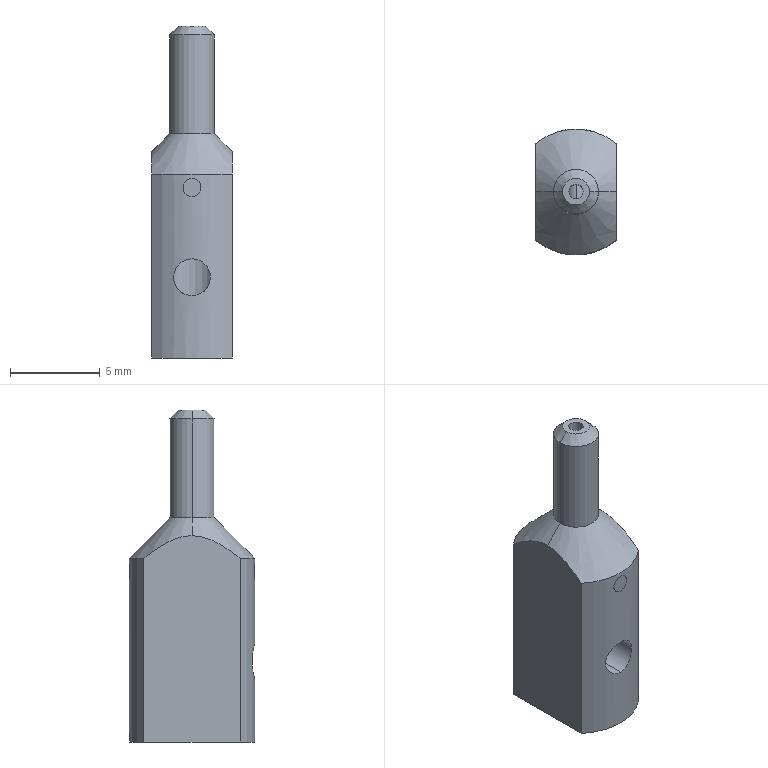Part | SolidWorks | features ICE 7, Chamfer 2, Extrusion 1, HoleWzd 1 | 2 solids | 27 faces | box 4.5 x 7 x 18.5 mm | volume 294.57 mm3 | cylinder 16 | plane 7 | cone 4 | commonest cylinder face diameters 0.8 x4 1 x4 2.05 x2 2.5 x2 3 x2 7 x2
STEP:
#1=CARTESIAN_POINT('',(0.,3.5,10.));
#2=VERTEX_POINT('',#1);
#3=CARTESIAN_POINT('',(0.,3.5,9.));
#4=VERTEX_POINT('',#3);
#5=CARTESIAN_POINT('',(0.,3.5,9.5));
#6=DIRECTION('',(0.,1.,0.));
#7=DIRECTION('',(0.,0.,1.));
#8=AXIS2_PLACEMENT_3D('',#5,#6,#7);
#9=CIRCLE('',#8,0.5);
#10=EDGE_CURVE('',#2,#4,#9,.T.);
#11=ORIENTED_EDGE('',*,*,#10,.F.);
#12=CARTESIAN_POINT('',(0.,-3.5,10.));
#13=VERTEX_POINT('',#12);
#14=CARTESIAN_POINT('',(0.,3.5,10.));
#15=DIRECTION('',(0.,-1.,0.));
#16=VECTOR('',#15,1000.);
#17=LINE('',#14,#16);
#18=EDGE_CURVE('',#2,#13,#17,.T.);
#19=ORIENTED_EDGE('',*,*,#18,.T.);
#20=CARTESIAN_POINT('',(0.,-3.5,9.));
#21=VERTEX_POINT('',#20);
#22=CARTESIAN_POINT('',(0.,-3.5,9.5));
#23=DIRECTION('',(0.,1.,0.));
#24=DIRECTION('',(0.,0.,1.));
#25=AXIS2_PLACEMENT_3D('',#22,#23,#24);
#26=CIRCLE('',#25,0.5);
#27=EDGE_CURVE('',#13,#21,#26,.T.);
#28=ORIENTED_EDGE('',*,*,#27,.T.);
#29=CARTESIAN_POINT('',(0.,3.5,9.));
#30=DIRECTION('',(0.,-1.,0.));
#31=VECTOR('',#30,1000.);
#32=LINE('',#29,#31);
#33=EDGE_CURVE('',#4,#21,#32,.T.);
#34=ORIENTED_EDGE('',*,*,#33,.F.);
#35=EDGE_LOOP('',(#11,#19,#28,#34));
#36=FACE_OUTER_BOUND('',#35,.T.);
#37=CARTESIAN_POINT('',(0.,3.5,9.5));
#38=DIRECTION('',(0.,-1.,0.));
#39=DIRECTION('',(0.,0.,-1.));
#40=AXIS2_PLACEMENT_3D('',#37,#38,#39);
#41=CYLINDRICAL_SURFACE('',#40,0.5);
#42=ADVANCED_FACE('',(#36),#41,.T.);
#43=ORIENTED_EDGE('',*,*,#18,.F.);
#44=CARTESIAN_POINT('',(0.,3.5,9.5));
#45=DIRECTION('',(0.,1.,0.));
#46=DIRECTION('',(0.,0.,1.));
#47=AXIS2_PLACEMENT_3D('',#44,#45,#46);
#48=CIRCLE('',#47,0.5);
#49=EDGE_CURVE('',#4,#2,#48,.T.);
#50=ORIENTED_EDGE('',*,*,#49,.F.);
#51=ORIENTED_EDGE('',*,*,#33,.T.);
#52=CARTESIAN_POINT('',(0.,-3.5,9.5));
#53=DIRECTION('',(0.,1.,0.));
#54=DIRECTION('',(0.,0.,1.));
#55=AXIS2_PLACEMENT_3D('',#52,#53,#54);
#56=CIRCLE('',#55,0.5);
#57=EDGE_CURVE('',#21,#13,#56,.T.);
#58=ORIENTED_EDGE('',*,*,#57,.T.);
#59=EDGE_LOOP('',(#43,#50,#51,#58));
#60=FACE_OUTER_BOUND('',#59,.T.);
#61=CARTESIAN_POINT('',(0.,3.5,9.5));
#62=DIRECTION('',(0.,-1.,0.));
#63=DIRECTION('',(0.,0.,-1.));
#64=AXIS2_PLACEMENT_3D('',#61,#62,#63);
#65=CYLINDRICAL_SURFACE('',#64,0.5);
#66=ADVANCED_FACE('',(#60),#65,.T.);
#67=ORIENTED_EDGE('',*,*,#49,.T.);
#68=ORIENTED_EDGE('',*,*,#10,.T.);
#69=EDGE_LOOP('',(#67,#68));
#70=FACE_OUTER_BOUND('',#69,.T.);
#71=CARTESIAN_POINT('',(0.,3.5,9.5));
#72=DIRECTION('',(0.,1.,0.));
#73=DIRECTION('',(0.,0.,1.));
#74=AXIS2_PLACEMENT_3D('',#71,#72,#73);
#75=PLANE('',#74);
#76=ADVANCED_FACE('',(#70),#75,.T.);
#77=ORIENTED_EDGE('',*,*,#57,.F.);
#78=ORIENTED_EDGE('',*,*,#27,.F.);
#79=EDGE_LOOP('',(#77,#78));
#80=FACE_OUTER_BOUND('',#79,.T.);
#81=CARTESIAN_POINT('',(0.,-3.5,9.5));
#82=DIRECTION('',(0.,1.,0.));
#83=DIRECTION('',(0.,0.,1.));
#84=AXIS2_PLACEMENT_3D('',#81,#82,#83);
#85=PLANE('',#84);
#86=ADVANCED_FACE('',(#80),#85,.F.);
#87=CLOSED_SHELL('',(#42,#66,#76,#86));
#88=MANIFOLD_SOLID_BREP('',#87);
#89=CARTESIAN_POINT('',(0.,-1.5,5.525));
#90=VERTEX_POINT('',#89);
#91=CARTESIAN_POINT('',(0.,-1.5,3.475));
#92=VERTEX_POINT('',#91);
#93=CARTESIAN_POINT('',(0.,-1.5,5.525));
#94=CARTESIAN_POINT('',(-0.1385,-1.5,5.525));
#95=CARTESIAN_POINT('',(-0.2773,-1.48,5.496));
#96=CARTESIAN_POINT('',(-0.5262,-1.411,5.39));
#97=CARTESIAN_POINT('',(-0.6364,-1.362,5.314));
#98=CARTESIAN_POINT('',(-0.8192,-1.261,5.13));
#99=CARTESIAN_POINT('',(-0.8927,-1.207,5.021));
#100=CARTESIAN_POINT('',(-0.9957,-1.124,4.777));
#101=CARTESIAN_POINT('',(-1.025,-1.095,4.639));
#102=CARTESIAN_POINT('',(-1.025,-1.095,4.36));
#103=CARTESIAN_POINT('',(-0.9952,-1.124,4.221));
#104=CARTESIAN_POINT('',(-0.8919,-1.208,3.978));
#105=CARTESIAN_POINT('',(-0.8179,-1.262,3.869));
#106=CARTESIAN_POINT('',(-0.6356,-1.363,3.686));
#107=CARTESIAN_POINT('',(-0.5254,-1.411,3.61));
#108=CARTESIAN_POINT('',(-0.2793,-1.479,3.505));
#109=CARTESIAN_POINT('',(-0.1404,-1.5,3.475));
#110=CARTESIAN_POINT('',(0.,-1.5,3.475));
#111=B_SPLINE_CURVE_WITH_KNOTS('',3,(#93,#94,#95,#96,#97,#98,#99,#100,#101,#102,#103,#104,#105,#106,#107,#108,#109,#110),.UNSPECIFIED.,.F.,.F.,(4,2,2,2,2,2,2,2,4),(0.003321,0.003736,0.00415,0.004565,0.004979,0.005394,0.005808,0.006223,0.006638),.UNSPECIFIED.);
#112=EDGE_CURVE('',#90,#92,#111,.T.);
#113=ORIENTED_EDGE('',*,*,#112,.F.);
#114=CARTESIAN_POINT('',(0.,-3.5,5.525));
#115=VERTEX_POINT('',#114);
#116=CARTESIAN_POINT('',(0.,-3.5,5.525));
#117=DIRECTION('',(0.,-1.,0.));
#118=VECTOR('',#117,1000.);
#119=LINE('',#116,#118);
#120=EDGE_CURVE('',#90,#115,#119,.T.);
#121=ORIENTED_EDGE('',*,*,#120,.T.);
#122=CARTESIAN_POINT('',(0.,-3.5,3.475));
#123=VERTEX_POINT('',#122);
#124=CARTESIAN_POINT('',(0.,-3.5,3.475));
#125=CARTESIAN_POINT('',(-0.1363,-3.5,3.475));
#126=CARTESIAN_POINT('',(-0.2699,-3.492,3.502));
#127=CARTESIAN_POINT('',(-0.5179,-3.464,3.605));
#128=CARTESIAN_POINT('',(-0.6311,-3.444,3.681));
#129=CARTESIAN_POINT('',(-0.819,-3.404,3.87));
#130=CARTESIAN_POINT('',(-0.8952,-3.384,3.983));
#131=CARTESIAN_POINT('',(-0.9977,-3.355,4.23));
#132=CARTESIAN_POINT('',(-1.025,-3.347,4.365));
#133=CARTESIAN_POINT('',(-1.025,-3.347,4.634));
#134=CARTESIAN_POINT('',(-0.9983,-3.355,4.769));
#135=CARTESIAN_POINT('',(-0.8948,-3.384,5.018));
#136=CARTESIAN_POINT('',(-0.8192,-3.404,5.13));
#137=CARTESIAN_POINT('',(-0.6299,-3.444,5.32));
#138=CARTESIAN_POINT('',(-0.5168,-3.464,5.395));
#139=CARTESIAN_POINT('',(-0.2696,-3.492,5.498));
#140=CARTESIAN_POINT('',(-0.1343,-3.5,5.525));
#141=CARTESIAN_POINT('',(0.,-3.5,5.525));
#142=B_SPLINE_CURVE_WITH_KNOTS('',3,(#124,#125,#126,#127,#128,#129,#130,#131,#132,#133,#134,#135,#136,#137,#138,#139,#140,#141),.UNSPECIFIED.,.F.,.F.,(4,2,2,2,2,2,2,2,4),(0.,0.0004028,0.0008056,0.001208,0.001611,0.002014,0.002417,0.00282,0.003222),.UNSPECIFIED.);
#143=EDGE_CURVE('',#123,#115,#142,.T.);
#144=ORIENTED_EDGE('',*,*,#143,.F.);
#145=CARTESIAN_POINT('',(0.,-3.5,3.475));
#146=DIRECTION('',(0.,-1.,0.));
#147=VECTOR('',#146,1000.);
#148=LINE('',#145,#147);
#149=EDGE_CURVE('',#92,#123,#148,.T.);
#150=ORIENTED_EDGE('',*,*,#149,.F.);
#151=EDGE_LOOP('',(#113,#121,#144,#150));
#152=FACE_OUTER_BOUND('',#151,.T.);
#153=CARTESIAN_POINT('',(0.,-3.5,4.5));
#154=DIRECTION('',(0.,-1.,0.));
#155=DIRECTION('',(0.,0.,-1.));
#156=AXIS2_PLACEMENT_3D('',#153,#154,#155);
#157=CYLINDRICAL_SURFACE('',#156,1.025);
#158=ADVANCED_FACE('',(#152),#157,.F.);
#159=CARTESIAN_POINT('',(0.75,0.,18.5));
#160=VERTEX_POINT('',#159);
#161=CARTESIAN_POINT('',(-0.75,0.,18.5));
#162=VERTEX_POINT('',#161);
#163=CARTESIAN_POINT('',(0.,0.,18.5));
#164=DIRECTION('',(0.,0.,1.));
#165=DIRECTION('',(1.,0.,0.));
#166=AXIS2_PLACEMENT_3D('',#163,#164,#165);
#167=CIRCLE('',#166,0.75);
#168=EDGE_CURVE('',#160,#162,#167,.T.);
#169=ORIENTED_EDGE('',*,*,#168,.F.);
#170=CARTESIAN_POINT('',(1.25,0.,18.));
#171=VERTEX_POINT('',#170);
#172=CARTESIAN_POINT('',(0.75,0.,18.5));
#173=DIRECTION('',(0.7071,0.,-0.7071));
#174=VECTOR('',#173,1000.);
#175=LINE('',#172,#174);
#176=EDGE_CURVE('',#160,#171,#175,.T.);
#177=ORIENTED_EDGE('',*,*,#176,.T.);
#178=CARTESIAN_POINT('',(-1.25,0.,18.));
#179=VERTEX_POINT('',#178);
#180=CARTESIAN_POINT('',(0.,0.,18.));
#181=DIRECTION('',(0.,0.,-1.));
#182=DIRECTION('',(1.,0.,0.));
#183=AXIS2_PLACEMENT_3D('',#180,#181,#182);
#184=CIRCLE('',#183,1.25);
#185=EDGE_CURVE('',#179,#171,#184,.T.);
#186=ORIENTED_EDGE('',*,*,#185,.F.);
#187=CARTESIAN_POINT('',(-0.75,0.,18.5));
#188=DIRECTION('',(-0.7071,0.,-0.7071));
#189=VECTOR('',#188,1000.);
#190=LINE('',#187,#189);
#191=EDGE_CURVE('',#162,#179,#190,.T.);
#192=ORIENTED_EDGE('',*,*,#191,.F.);
#193=EDGE_LOOP('',(#169,#177,#186,#192));
#194=FACE_OUTER_BOUND('',#193,.T.);
#195=CARTESIAN_POINT('',(0.,0.,18.5));
#196=DIRECTION('',(0.,0.,-1.));
#197=DIRECTION('',(-1.,0.,0.));
#198=AXIS2_PLACEMENT_3D('',#195,#196,#197);
#199=CONICAL_SURFACE('',#198,0.75,0.7854);
#200=ADVANCED_FACE('',(#194),#199,.T.);
#201=CARTESIAN_POINT('',(0.,-3.5,9.));
#202=VERTEX_POINT('',#201);
#203=CARTESIAN_POINT('',(0.,-3.5,10.));
#204=VERTEX_POINT('',#203);
#205=CARTESIAN_POINT('',(0.,-3.5,9.));
#206=CARTESIAN_POINT('',(-0.1306,-3.5,9.));
#207=CARTESIAN_POINT('',(-0.2611,-3.491,9.054));
#208=CARTESIAN_POINT('',(-0.4456,-3.473,9.238));
#209=CARTESIAN_POINT('',(-0.4999,-3.464,9.367));
#210=CARTESIAN_POINT('',(-0.5001,-3.464,9.632));
#211=CARTESIAN_POINT('',(-0.4458,-3.473,9.761));
#212=CARTESIAN_POINT('',(-0.2618,-3.491,9.945));
#213=CARTESIAN_POINT('',(-0.1323,-3.5,10.));
#214=CARTESIAN_POINT('',(0.,-3.5,10.));
#215=B_SPLINE_CURVE_WITH_KNOTS('',3,(#205,#206,#207,#208,#209,#210,#211,#212,#213,#214),.UNSPECIFIED.,.F.,.F.,(4,2,2,2,4),(0.001565,0.001956,0.002348,0.002739,0.00313),.UNSPECIFIED.);
#216=EDGE_CURVE('',#202,#204,#215,.T.);
#217=ORIENTED_EDGE('',*,*,#216,.F.);
#218=CARTESIAN_POINT('',(0.,-0.4,9.));
#219=VERTEX_POINT('',#218);
#220=CARTESIAN_POINT('',(0.,-4.,9.));
#221=DIRECTION('',(0.,1.,0.));
#222=VECTOR('',#221,1000.);
#223=LINE('',#220,#222);
#224=EDGE_CURVE('',#202,#219,#223,.T.);
#225=ORIENTED_EDGE('',*,*,#224,.T.);
#226=CARTESIAN_POINT('',(-0.4,0.,9.2));
#227=VERTEX_POINT('',#226);
#228=CARTESIAN_POINT('',(-0.4,0.,9.2));
#229=CARTESIAN_POINT('',(-0.4,-0.05567,9.2));
#230=CARTESIAN_POINT('',(-0.3881,-0.1095,9.183));
#231=CARTESIAN_POINT('',(-0.348,-0.2038,9.14));
#232=CARTESIAN_POINT('',(-0.3203,-0.2447,9.114));
#233=CARTESIAN_POINT('',(-0.2501,-0.3161,9.065));
#234=CARTESIAN_POINT('',(-0.2086,-0.3454,9.043));
#235=CARTESIAN_POINT('',(-0.1109,-0.388,9.01));
#236=CARTESIAN_POINT('',(-0.05536,-0.4,9.));
#237=CARTESIAN_POINT('',(0.,-0.4,9.));
#238=B_SPLINE_CURVE_WITH_KNOTS('',3,(#228,#229,#230,#231,#232,#233,#234,#235,#236,#237),.UNSPECIFIED.,.F.,.F.,(4,2,2,2,4),(0.001327,0.001493,0.001659,0.001825,0.001991),.UNSPECIFIED.);
#239=EDGE_CURVE('',#227,#219,#238,.T.);
#240=ORIENTED_EDGE('',*,*,#239,.F.);
#241=CARTESIAN_POINT('',(0.,0.4,9.));
#242=VERTEX_POINT('',#241);
#243=CARTESIAN_POINT('',(0.,0.4,9.));
#244=CARTESIAN_POINT('',(-0.05517,0.4,9.));
#245=CARTESIAN_POINT('',(-0.1102,0.3882,9.01));
#246=CARTESIAN_POINT('',(-0.2079,0.3458,9.042));
#247=CARTESIAN_POINT('',(-0.2503,0.3159,9.065));
#248=CARTESIAN_POINT('',(-0.3201,0.2449,9.114));
#249=CARTESIAN_POINT('',(-0.3481,0.2035,9.14));
#250=CARTESIAN_POINT('',(-0.3879,0.11,9.183));
#251=CARTESIAN_POINT('',(-0.4,0.05556,9.2));
#252=CARTESIAN_POINT('',(-0.4,0.,9.2));
#253=B_SPLINE_CURVE_WITH_KNOTS('',3,(#243,#244,#245,#246,#247,#248,#249,#250,#251,#252),.UNSPECIFIED.,.F.,.F.,(4,2,2,2,4),(0.000664,0.0008296,0.0009953,0.001161,0.001327),.UNSPECIFIED.);
#254=EDGE_CURVE('',#242,#227,#253,.T.);
#255=ORIENTED_EDGE('',*,*,#254,.F.);
#256=CARTESIAN_POINT('',(0.,3.5,9.));
#257=VERTEX_POINT('',#256);
#258=CARTESIAN_POINT('',(0.,-4.,9.));
#259=DIRECTION('',(0.,1.,0.));
#260=VECTOR('',#259,1000.);
#261=LINE('',#258,#260);
#262=EDGE_CURVE('',#242,#257,#261,.T.);
#263=ORIENTED_EDGE('',*,*,#262,.T.);
#264=CARTESIAN_POINT('',(0.,3.5,10.));
#265=VERTEX_POINT('',#264);
#266=CARTESIAN_POINT('',(0.,3.5,10.));
#267=CARTESIAN_POINT('',(-0.1323,3.5,10.));
#268=CARTESIAN_POINT('',(-0.2615,3.491,9.946));
#269=CARTESIAN_POINT('',(-0.4457,3.473,9.761));
#270=CARTESIAN_POINT('',(-0.5,3.464,9.631));
#271=CARTESIAN_POINT('',(-0.5,3.464,9.37));
#272=CARTESIAN_POINT('',(-0.4468,3.473,9.24));
#273=CARTESIAN_POINT('',(-0.2604,3.492,9.053));
#274=CARTESIAN_POINT('',(-0.1306,3.5,9.));
#275=CARTESIAN_POINT('',(0.,3.5,9.));
#276=B_SPLINE_CURVE_WITH_KNOTS('',3,(#266,#267,#268,#269,#270,#271,#272,#273,#274,#275),.UNSPECIFIED.,.F.,.F.,(4,2,2,2,4),(0.,0.0003913,0.0007826,0.001174,0.001565),.UNSPECIFIED.);
#277=EDGE_CURVE('',#265,#257,#276,.T.);
#278=ORIENTED_EDGE('',*,*,#277,.F.);
#279=CARTESIAN_POINT('',(0.,0.4,10.));
#280=VERTEX_POINT('',#279);
#281=CARTESIAN_POINT('',(0.,-4.,10.));
#282=DIRECTION('',(0.,1.,0.));
#283=VECTOR('',#282,1000.);
#284=LINE('',#281,#283);
#285=EDGE_CURVE('',#280,#265,#284,.T.);
#286=ORIENTED_EDGE('',*,*,#285,.F.);
#287=CARTESIAN_POINT('',(-0.4,0.,9.8));
#288=VERTEX_POINT('',#287);
#289=CARTESIAN_POINT('',(-0.4,0.,9.8));
#290=CARTESIAN_POINT('',(-0.4,0.05567,9.8));
#291=CARTESIAN_POINT('',(-0.3881,0.1095,9.817));
#292=CARTESIAN_POINT('',(-0.348,0.2038,9.86));
#293=CARTESIAN_POINT('',(-0.3203,0.2447,9.886));
#294=CARTESIAN_POINT('',(-0.2501,0.3161,9.935));
#295=CARTESIAN_POINT('',(-0.2086,0.3454,9.957));
#296=CARTESIAN_POINT('',(-0.1109,0.388,9.99));
#297=CARTESIAN_POINT('',(-0.05536,0.4,10.));
#298=CARTESIAN_POINT('',(0.,0.4,10.));
#299=B_SPLINE_CURVE_WITH_KNOTS('',3,(#289,#290,#291,#292,#293,#294,#295,#296,#297,#298),.UNSPECIFIED.,.F.,.F.,(4,2,2,2,4),(0.001327,0.001493,0.001659,0.001825,0.001991),.UNSPECIFIED.);
#300=EDGE_CURVE('',#288,#280,#299,.T.);
#301=ORIENTED_EDGE('',*,*,#300,.F.);
#302=CARTESIAN_POINT('',(0.,-0.4,10.));
#303=VERTEX_POINT('',#302);
#304=CARTESIAN_POINT('',(0.,-0.4,10.));
#305=CARTESIAN_POINT('',(-0.05517,-0.4,10.));
#306=CARTESIAN_POINT('',(-0.1102,-0.3882,9.99));
#307=CARTESIAN_POINT('',(-0.2079,-0.3458,9.958));
#308=CARTESIAN_POINT('',(-0.2503,-0.3159,9.935));
#309=CARTESIAN_POINT('',(-0.3201,-0.2449,9.886));
#310=CARTESIAN_POINT('',(-0.3481,-0.2035,9.86));
#311=CARTESIAN_POINT('',(-0.3879,-0.11,9.817));
#312=CARTESIAN_POINT('',(-0.4,-0.05556,9.8));
#313=CARTESIAN_POINT('',(-0.4,0.,9.8));
#314=B_SPLINE_CURVE_WITH_KNOTS('',3,(#304,#305,#306,#307,#308,#309,#310,#311,#312,#313),.UNSPECIFIED.,.F.,.F.,(4,2,2,2,4),(0.000664,0.0008296,0.0009953,0.001161,0.001327),.UNSPECIFIED.);
#315=EDGE_CURVE('',#303,#288,#314,.T.);
#316=ORIENTED_EDGE('',*,*,#315,.F.);
#317=CARTESIAN_POINT('',(0.,-4.,10.));
#318=DIRECTION('',(0.,1.,0.));
#319=VECTOR('',#318,1000.);
#320=LINE('',#317,#319);
#321=EDGE_CURVE('',#204,#303,#320,.T.);
#322=ORIENTED_EDGE('',*,*,#321,.F.);
#323=EDGE_LOOP('',(#217,#225,#240,#255,#263,#278,#286,#301,#316,#322));
#324=FACE_OUTER_BOUND('',#323,.T.);
#325=CARTESIAN_POINT('',(0.,-4.,9.5));
#326=DIRECTION('',(0.,1.,0.));
#327=DIRECTION('',(0.,0.,1.));
#328=AXIS2_PLACEMENT_3D('',#325,#326,#327);
#329=CYLINDRICAL_SURFACE('',#328,0.5);
#330=ADVANCED_FACE('',(#324),#329,.F.);
#331=CARTESIAN_POINT('',(0.,-1.5,3.475));
#332=CARTESIAN_POINT('',(0.1406,-1.5,3.475));
#333=CARTESIAN_POINT('',(0.2781,-1.48,3.504));
#334=CARTESIAN_POINT('',(0.5256,-1.411,3.61));
#335=CARTESIAN_POINT('',(0.6359,-1.363,3.686));
#336=CARTESIAN_POINT('',(0.8184,-1.261,3.869));
#337=CARTESIAN_POINT('',(0.8918,-1.208,3.978));
#338=CARTESIAN_POINT('',(0.9953,-1.124,4.222));
#339=CARTESIAN_POINT('',(1.025,-1.095,4.36));
#340=CARTESIAN_POINT('',(1.025,-1.095,4.639));
#341=CARTESIAN_POINT('',(0.996,-1.124,4.777));
#342=CARTESIAN_POINT('',(0.8921,-1.208,5.022));
#343=CARTESIAN_POINT('',(0.8193,-1.261,5.13));
#344=CARTESIAN_POINT('',(0.6355,-1.363,5.315));
#345=CARTESIAN_POINT('',(0.5275,-1.41,5.389));
#346=CARTESIAN_POINT('',(0.3399,-1.462,5.469));
#347=CARTESIAN_POINT('',(0.2749,-1.476,5.49));
#348=CARTESIAN_POINT('',(0.1398,-1.495,5.518));
#349=CARTESIAN_POINT('',(0.06933,-1.5,5.525));
#350=CARTESIAN_POINT('',(0.,-1.5,5.525));
#351=B_SPLINE_CURVE_WITH_KNOTS('',3,(#331,#332,#333,#334,#335,#336,#337,#338,#339,#340,#341,#342,#343,#344,#345,#346,#347,#348,#349,#350),.UNSPECIFIED.,.F.,.F.,(4,2,2,2,2,2,2,2,2,4),(0.,0.0004152,0.0008303,0.001245,0.001661,0.002076,0.002491,0.002906,0.003114,0.003321),.UNSPECIFIED.);
#352=EDGE_CURVE('',#92,#90,#351,.T.);
#353=ORIENTED_EDGE('',*,*,#352,.T.);
#354=ORIENTED_EDGE('',*,*,#112,.T.);
#355=EDGE_LOOP('',(#353,#354));
#356=FACE_BOUND('',#355,.T.);
#357=CARTESIAN_POINT('',(1.5,0.,8.5));
#358=VERTEX_POINT('',#357);
#359=CARTESIAN_POINT('',(-1.5,0.,8.5));
#360=VERTEX_POINT('',#359);
#361=CARTESIAN_POINT('',(0.,0.,8.5));
#362=DIRECTION('',(0.,0.,-1.));
#363=DIRECTION('',(-1.,0.,0.));
#364=AXIS2_PLACEMENT_3D('',#361,#362,#363);
#365=CIRCLE('',#364,1.5);
#366=EDGE_CURVE('',#358,#360,#365,.T.);
#367=ORIENTED_EDGE('',*,*,#366,.F.);
#368=CARTESIAN_POINT('',(1.5,0.,0.));
#369=VERTEX_POINT('',#368);
#370=CARTESIAN_POINT('',(1.5,0.,8.5));
#371=DIRECTION('',(0.,0.,-1.));
#372=VECTOR('',#371,1000.);
#373=LINE('',#370,#372);
#374=EDGE_CURVE('',#358,#369,#373,.T.);
#375=ORIENTED_EDGE('',*,*,#374,.T.);
#376=CARTESIAN_POINT('',(-1.5,0.,0.));
#377=VERTEX_POINT('',#376);
#378=CARTESIAN_POINT('',(0.,0.,0.));
#379=DIRECTION('',(0.,0.,-1.));
#380=DIRECTION('',(-1.,0.,0.));
#381=AXIS2_PLACEMENT_3D('',#378,#379,#380);
#382=CIRCLE('',#381,1.5);
#383=EDGE_CURVE('',#369,#377,#382,.T.);
#384=ORIENTED_EDGE('',*,*,#383,.T.);
#385=CARTESIAN_POINT('',(-1.5,0.,8.5));
#386=DIRECTION('',(0.,0.,-1.));
#387=VECTOR('',#386,1000.);
#388=LINE('',#385,#387);
#389=EDGE_CURVE('',#360,#377,#388,.T.);
#390=ORIENTED_EDGE('',*,*,#389,.F.);
#391=EDGE_LOOP('',(#367,#375,#384,#390));
#392=FACE_OUTER_BOUND('',#391,.T.);
#393=CARTESIAN_POINT('',(0.,0.,8.5));
#394=DIRECTION('',(0.,0.,-1.));
#395=DIRECTION('',(-1.,0.,0.));
#396=AXIS2_PLACEMENT_3D('',#393,#394,#395);
#397=CYLINDRICAL_SURFACE('',#396,1.5);
#398=ADVANCED_FACE('',(#356,#392),#397,.F.);
#399=ORIENTED_EDGE('',*,*,#185,.T.);
#400=CARTESIAN_POINT('',(1.25,0.,12.5));
#401=VERTEX_POINT('',#400);
#402=CARTESIAN_POINT('',(1.25,0.,18.5));
#403=DIRECTION('',(0.,0.,-1.));
#404=VECTOR('',#403,1000.);
#405=LINE('',#402,#404);
#406=EDGE_CURVE('',#171,#401,#405,.T.);
#407=ORIENTED_EDGE('',*,*,#406,.T.);
#408=CARTESIAN_POINT('',(-1.25,0.,12.5));
#409=VERTEX_POINT('',#408);
#410=CARTESIAN_POINT('',(0.,0.,12.5));
#411=DIRECTION('',(0.,0.,1.));
#412=DIRECTION('',(1.,0.,0.));
#413=AXIS2_PLACEMENT_3D('',#410,#411,#412);
#414=CIRCLE('',#413,1.25);
#415=EDGE_CURVE('',#401,#409,#414,.T.);
#416=ORIENTED_EDGE('',*,*,#415,.T.);
#417=CARTESIAN_POINT('',(-1.25,0.,18.5));
#418=DIRECTION('',(0.,0.,-1.));
#419=VECTOR('',#418,1000.);
#420=LINE('',#417,#419);
#421=EDGE_CURVE('',#179,#409,#420,.T.);
#422=ORIENTED_EDGE('',*,*,#421,.F.);
#423=EDGE_LOOP('',(#399,#407,#416,#422));
#424=FACE_OUTER_BOUND('',#423,.T.);
#425=CARTESIAN_POINT('',(0.,0.,18.5));
#426=DIRECTION('',(0.,0.,-1.));
#427=DIRECTION('',(-1.,0.,0.));
#428=AXIS2_PLACEMENT_3D('',#425,#426,#427);
#429=CYLINDRICAL_SURFACE('',#428,1.25);
#430=ADVANCED_FACE('',(#424),#429,.T.);
#431=CARTESIAN_POINT('',(0.4,0.,9.8));
#432=VERTEX_POINT('',#431);
#433=CARTESIAN_POINT('',(0.4,0.,9.8));
#434=CARTESIAN_POINT('',(0.4,-0.05624,9.8));
#435=CARTESIAN_POINT('',(0.388,-0.1098,9.817));
#436=CARTESIAN_POINT('',(0.3481,-0.2035,9.86));
#437=CARTESIAN_POINT('',(0.3202,-0.2449,9.886));
#438=CARTESIAN_POINT('',(0.2506,-0.3157,9.935));
#439=CARTESIAN_POINT('',(0.2083,-0.3456,9.957));
#440=CARTESIAN_POINT('',(0.1107,-0.3881,9.99));
#441=CARTESIAN_POINT('',(0.05527,-0.4,10.));
#442=CARTESIAN_POINT('',(0.,-0.4,10.));
#443=B_SPLINE_CURVE_WITH_KNOTS('',3,(#433,#434,#435,#436,#437,#438,#439,#440,#441,#442),.UNSPECIFIED.,.F.,.F.,(4,2,2,2,4),(0.,0.000166,0.000332,0.000498,0.000664),.UNSPECIFIED.);
#444=EDGE_CURVE('',#432,#303,#443,.T.);
#445=ORIENTED_EDGE('',*,*,#444,.T.);
#446=ORIENTED_EDGE('',*,*,#315,.T.);
#447=CARTESIAN_POINT('',(-0.4,0.,18.5));
#448=VERTEX_POINT('',#447);
#449=CARTESIAN_POINT('',(-0.4,0.,-2.5));
#450=DIRECTION('',(0.,0.,1.));
#451=VECTOR('',#450,1000.);
#452=LINE('',#449,#451);
#453=EDGE_CURVE('',#288,#448,#452,.T.);
#454=ORIENTED_EDGE('',*,*,#453,.T.);
#455=CARTESIAN_POINT('',(0.4,0.,18.5));
#456=VERTEX_POINT('',#455);
#457=CARTESIAN_POINT('',(0.,0.,18.5));
#458=DIRECTION('',(0.,0.,1.));
#459=DIRECTION('',(1.,0.,0.));
#460=AXIS2_PLACEMENT_3D('',#457,#458,#459);
#461=CIRCLE('',#460,0.4);
#462=EDGE_CURVE('',#448,#456,#461,.T.);
#463=ORIENTED_EDGE('',*,*,#462,.T.);
#464=CARTESIAN_POINT('',(0.4,0.,-2.5));
#465=DIRECTION('',(0.,0.,1.));
#466=VECTOR('',#465,1000.);
#467=LINE('',#464,#466);
#468=EDGE_CURVE('',#432,#456,#467,.T.);
#469=ORIENTED_EDGE('',*,*,#468,.F.);
#470=EDGE_LOOP('',(#445,#446,#454,#463,#469));
#471=FACE_OUTER_BOUND('',#470,.T.);
#472=CARTESIAN_POINT('',(0.,0.,-2.5));
#473=DIRECTION('',(0.,0.,1.));
#474=DIRECTION('',(1.,0.,0.));
#475=AXIS2_PLACEMENT_3D('',#472,#473,#474);
#476=CYLINDRICAL_SURFACE('',#475,0.4);
#477=ADVANCED_FACE('',(#471),#476,.F.);
#478=CARTESIAN_POINT('',(-0.4,0.,8.5));
#479=VERTEX_POINT('',#478);
#480=CARTESIAN_POINT('',(0.4,0.,8.5));
#481=VERTEX_POINT('',#480);
#482=CARTESIAN_POINT('',(0.,0.,8.5));
#483=DIRECTION('',(0.,0.,1.));
#484=DIRECTION('',(-1.,0.,0.));
#485=AXIS2_PLACEMENT_3D('',#482,#483,#484);
#486=CIRCLE('',#485,0.4);
#487=EDGE_CURVE('',#479,#481,#486,.T.);
#488=ORIENTED_EDGE('',*,*,#487,.F.);
#489=CARTESIAN_POINT('',(-0.4,0.,-2.5));
#490=DIRECTION('',(0.,0.,1.));
#491=VECTOR('',#490,1000.);
#492=LINE('',#489,#491);
#493=EDGE_CURVE('',#479,#227,#492,.T.);
#494=ORIENTED_EDGE('',*,*,#493,.T.);
#495=ORIENTED_EDGE('',*,*,#239,.T.);
#496=CARTESIAN_POINT('',(0.4,0.,9.2));
#497=VERTEX_POINT('',#496);
#498=CARTESIAN_POINT('',(0.,-0.4,9.));
#499=CARTESIAN_POINT('',(0.05515,-0.4,9.));
#500=CARTESIAN_POINT('',(0.1102,-0.3882,9.01));
#501=CARTESIAN_POINT('',(0.208,-0.3458,9.042));
#502=CARTESIAN_POINT('',(0.2503,-0.3159,9.065));
#503=CARTESIAN_POINT('',(0.3201,-0.245,9.114));
#504=CARTESIAN_POINT('',(0.3481,-0.2035,9.14));
#505=CARTESIAN_POINT('',(0.3879,-0.11,9.183));
#506=CARTESIAN_POINT('',(0.4,-0.05604,9.2));
#507=CARTESIAN_POINT('',(0.4,0.,9.2));
#508=B_SPLINE_CURVE_WITH_KNOTS('',3,(#498,#499,#500,#501,#502,#503,#504,#505,#506,#507),.UNSPECIFIED.,.F.,.F.,(4,2,2,2,4),(0.001991,0.002156,0.002322,0.002487,0.002652),.UNSPECIFIED.);
#509=EDGE_CURVE('',#219,#497,#508,.T.);
#510=ORIENTED_EDGE('',*,*,#509,.T.);
#511=CARTESIAN_POINT('',(0.4,0.,-2.5));
#512=DIRECTION('',(0.,0.,1.));
#513=VECTOR('',#512,1000.);
#514=LINE('',#511,#513);
#515=EDGE_CURVE('',#481,#497,#514,.T.);
#516=ORIENTED_EDGE('',*,*,#515,.F.);
#517=EDGE_LOOP('',(#488,#494,#495,#510,#516));
#518=FACE_OUTER_BOUND('',#517,.T.);
#519=CARTESIAN_POINT('',(0.,0.,-2.5));
#520=DIRECTION('',(0.,0.,1.));
#521=DIRECTION('',(1.,0.,0.));
#522=AXIS2_PLACEMENT_3D('',#519,#520,#521);
#523=CYLINDRICAL_SURFACE('',#522,0.4);
#524=ADVANCED_FACE('',(#518),#523,.F.);
#525=ORIENTED_EDGE('',*,*,#415,.F.);
#526=CARTESIAN_POINT('',(2.25,0.,11.5));
#527=VERTEX_POINT('',#526);
#528=CARTESIAN_POINT('',(1.25,0.,12.5));
#529=DIRECTION('',(0.7071,0.,-0.7071));
#530=VECTOR('',#529,1000.);
#531=LINE('',#528,#530);
#532=EDGE_CURVE('',#401,#527,#531,.T.);
#533=ORIENTED_EDGE('',*,*,#532,.T.);
#534=CARTESIAN_POINT('',(2.25,2.681,10.25));
#535=VERTEX_POINT('',#534);
#536=CARTESIAN_POINT('',(2.25,0.,11.5));
#537=CARTESIAN_POINT('',(2.25,0.1267,11.5));
#538=CARTESIAN_POINT('',(2.25,0.2541,11.489));
#539=CARTESIAN_POINT('',(2.25,0.5017,11.448));
#540=CARTESIAN_POINT('',(2.25,0.6232,11.418));
#541=CARTESIAN_POINT('',(2.25,0.9823,11.305));
#542=CARTESIAN_POINT('',(2.25,1.215,11.2));
#543=CARTESIAN_POINT('',(2.25,1.877,10.844));
#544=CARTESIAN_POINT('',(2.25,2.284,10.554));
#545=CARTESIAN_POINT('',(2.25,2.681,10.25));
#546=B_SPLINE_CURVE_WITH_KNOTS('',3,(#536,#537,#538,#539,#540,#541,#542,#543,#544,#545),.UNSPECIFIED.,.F.,.F.,(4,2,2,2,4),(0.007021,0.007397,0.007773,0.008524,0.01003),.UNSPECIFIED.);
#547=EDGE_CURVE('',#527,#535,#546,.T.);
#548=ORIENTED_EDGE('',*,*,#547,.T.);
#549=CARTESIAN_POINT('',(-2.25,2.681,10.25));
#550=VERTEX_POINT('',#549);
#551=CARTESIAN_POINT('',(0.,0.,10.25));
#552=DIRECTION('',(0.,0.,-1.));
#553=DIRECTION('',(1.,0.,0.));
#554=AXIS2_PLACEMENT_3D('',#551,#552,#553);
#555=CIRCLE('',#554,3.5);
#556=EDGE_CURVE('',#550,#535,#555,.T.);
#557=ORIENTED_EDGE('',*,*,#556,.F.);
#558=CARTESIAN_POINT('',(-2.25,0.,11.5));
#559=VERTEX_POINT('',#558);
#560=CARTESIAN_POINT('',(-2.25,2.681,10.25));
#561=CARTESIAN_POINT('',(-2.25,2.284,10.554));
#562=CARTESIAN_POINT('',(-2.25,1.877,10.844));
#563=CARTESIAN_POINT('',(-2.25,1.215,11.2));
#564=CARTESIAN_POINT('',(-2.25,0.9823,11.305));
#565=CARTESIAN_POINT('',(-2.25,0.6232,11.418));
#566=CARTESIAN_POINT('',(-2.25,0.5017,11.448));
#567=CARTESIAN_POINT('',(-2.25,0.2541,11.489));
#568=CARTESIAN_POINT('',(-2.25,0.1267,11.5));
#569=CARTESIAN_POINT('',(-2.25,0.,11.5));
#570=B_SPLINE_CURVE_WITH_KNOTS('',3,(#560,#561,#562,#563,#564,#565,#566,#567,#568,#569),.UNSPECIFIED.,.F.,.F.,(4,2,2,2,4),(0.01222,0.01372,0.01447,0.01484,0.01522),.UNSPECIFIED.);
#571=EDGE_CURVE('',#550,#559,#570,.T.);
#572=ORIENTED_EDGE('',*,*,#571,.T.);
#573=CARTESIAN_POINT('',(-1.25,0.,12.5));
#574=DIRECTION('',(-0.7071,0.,-0.7071));
#575=VECTOR('',#574,1000.);
#576=LINE('',#573,#575);
#577=EDGE_CURVE('',#409,#559,#576,.T.);
#578=ORIENTED_EDGE('',*,*,#577,.F.);
#579=EDGE_LOOP('',(#525,#533,#548,#557,#572,#578));
#580=FACE_OUTER_BOUND('',#579,.T.);
#581=CARTESIAN_POINT('',(0.,0.,12.5));
#582=DIRECTION('',(0.,0.,-1.));
#583=DIRECTION('',(-1.,0.,0.));
#584=AXIS2_PLACEMENT_3D('',#581,#582,#583);
#585=CONICAL_SURFACE('',#584,1.25,0.7854);
#586=ADVANCED_FACE('',(#580),#585,.T.);
#587=ORIENTED_EDGE('',*,*,#277,.T.);
#588=CARTESIAN_POINT('',(0.,3.5,9.));
#589=CARTESIAN_POINT('',(0.1306,3.5,9.));
#590=CARTESIAN_POINT('',(0.2611,3.491,9.054));
#591=CARTESIAN_POINT('',(0.4456,3.473,9.238));
#592=CARTESIAN_POINT('',(0.4999,3.464,9.367));
#593=CARTESIAN_POINT('',(0.5001,3.464,9.632));
#594=CARTESIAN_POINT('',(0.4458,3.473,9.761));
#595=CARTESIAN_POINT('',(0.2618,3.491,9.945));
#596=CARTESIAN_POINT('',(0.1323,3.5,10.));
#597=CARTESIAN_POINT('',(0.,3.5,10.));
#598=B_SPLINE_CURVE_WITH_KNOTS('',3,(#588,#589,#590,#591,#592,#593,#594,#595,#596,#597),.UNSPECIFIED.,.F.,.F.,(4,2,2,2,4),(0.001565,0.001956,0.002348,0.002739,0.00313),.UNSPECIFIED.);
#599=EDGE_CURVE('',#257,#265,#598,.T.);
#600=ORIENTED_EDGE('',*,*,#599,.T.);
#601=EDGE_LOOP('',(#587,#600));
#602=FACE_BOUND('',#601,.T.);
#603=CARTESIAN_POINT('',(-2.25,2.681,0.));
#604=VERTEX_POINT('',#603);
#605=CARTESIAN_POINT('',(-2.25,2.681,12.5));
#606=DIRECTION('',(0.,0.,-1.));
#607=VECTOR('',#606,1000.);
#608=LINE('',#605,#607);
#609=EDGE_CURVE('',#550,#604,#608,.T.);
#610=ORIENTED_EDGE('',*,*,#609,.F.);
#611=ORIENTED_EDGE('',*,*,#556,.T.);
#612=CARTESIAN_POINT('',(2.25,2.681,0.));
#613=VERTEX_POINT('',#612);
#614=CARTESIAN_POINT('',(2.25,2.681,12.5));
#615=DIRECTION('',(0.,0.,1.));
#616=VECTOR('',#615,1000.);
#617=LINE('',#614,#616);
#618=EDGE_CURVE('',#613,#535,#617,.T.);
#619=ORIENTED_EDGE('',*,*,#618,.F.);
#620=CARTESIAN_POINT('',(0.,0.,0.));
#621=DIRECTION('',(0.,0.,1.));
#622=DIRECTION('',(1.,0.,0.));
#623=AXIS2_PLACEMENT_3D('',#620,#621,#622);
#624=CIRCLE('',#623,3.5);
#625=EDGE_CURVE('',#613,#604,#624,.T.);
#626=ORIENTED_EDGE('',*,*,#625,.T.);
#627=EDGE_LOOP('',(#610,#611,#619,#626));
#628=FACE_OUTER_BOUND('',#627,.T.);
#629=CARTESIAN_POINT('',(0.,0.,12.5));
#630=DIRECTION('',(0.,0.,-1.));
#631=DIRECTION('',(-1.,0.,0.));
#632=AXIS2_PLACEMENT_3D('',#629,#630,#631);
#633=CYLINDRICAL_SURFACE('',#632,3.5);
#634=ADVANCED_FACE('',(#602,#628),#633,.T.);
#635=ORIENTED_EDGE('',*,*,#143,.T.);
#636=CARTESIAN_POINT('',(0.,-3.5,5.525));
#637=CARTESIAN_POINT('',(0.1342,-3.5,5.525));
#638=CARTESIAN_POINT('',(0.2698,-3.492,5.498));
#639=CARTESIAN_POINT('',(0.5169,-3.464,5.395));
#640=CARTESIAN_POINT('',(0.6301,-3.444,5.319));
#641=CARTESIAN_POINT('',(0.8192,-3.404,5.13));
#642=CARTESIAN_POINT('',(0.8944,-3.384,5.019));
#643=CARTESIAN_POINT('',(0.9984,-3.355,4.769));
#644=CARTESIAN_POINT('',(1.025,-3.347,4.635));
#645=CARTESIAN_POINT('',(1.025,-3.347,4.365));
#646=CARTESIAN_POINT('',(0.9978,-3.355,4.23));
#647=CARTESIAN_POINT('',(0.8952,-3.384,3.983));
#648=CARTESIAN_POINT('',(0.819,-3.404,3.87));
#649=CARTESIAN_POINT('',(0.6312,-3.444,3.682));
#650=CARTESIAN_POINT('',(0.5178,-3.464,3.605));
#651=CARTESIAN_POINT('',(0.2707,-3.492,3.502));
#652=CARTESIAN_POINT('',(0.1362,-3.5,3.475));
#653=CARTESIAN_POINT('',(0.,-3.5,3.475));
#654=B_SPLINE_CURVE_WITH_KNOTS('',3,(#636,#637,#638,#639,#640,#641,#642,#643,#644,#645,#646,#647,#648,#649,#650,#651,#652,#653),.UNSPECIFIED.,.F.,.F.,(4,2,2,2,2,2,2,2,4),(0.003222,0.003625,0.004028,0.00443,0.004833,0.005236,0.005638,0.006041,0.006444),.UNSPECIFIED.);
#655=EDGE_CURVE('',#115,#123,#654,.T.);
#656=ORIENTED_EDGE('',*,*,#655,.T.);
#657=EDGE_LOOP('',(#635,#656));
#658=FACE_BOUND('',#657,.T.);
#659=CARTESIAN_POINT('',(0.,-3.5,10.));
#660=CARTESIAN_POINT('',(0.1323,-3.5,10.));
#661=CARTESIAN_POINT('',(0.2615,-3.491,9.946));
#662=CARTESIAN_POINT('',(0.4457,-3.473,9.761));
#663=CARTESIAN_POINT('',(0.5,-3.464,9.631));
#664=CARTESIAN_POINT('',(0.5,-3.464,9.37));
#665=CARTESIAN_POINT('',(0.4468,-3.473,9.24));
#666=CARTESIAN_POINT('',(0.2604,-3.492,9.053));
#667=CARTESIAN_POINT('',(0.1306,-3.5,9.));
#668=CARTESIAN_POINT('',(0.,-3.5,9.));
#669=B_SPLINE_CURVE_WITH_KNOTS('',3,(#659,#660,#661,#662,#663,#664,#665,#666,#667,#668),.UNSPECIFIED.,.F.,.F.,(4,2,2,2,4),(0.,0.0003913,0.0007826,0.001174,0.001565),.UNSPECIFIED.);
#670=EDGE_CURVE('',#204,#202,#669,.T.);
#671=ORIENTED_EDGE('',*,*,#670,.T.);
#672=ORIENTED_EDGE('',*,*,#216,.T.);
#673=EDGE_LOOP('',(#671,#672));
#674=FACE_BOUND('',#673,.T.);
#675=CARTESIAN_POINT('',(-2.25,-2.681,0.));
#676=VERTEX_POINT('',#675);
#677=CARTESIAN_POINT('',(-2.25,-2.681,10.25));
#678=VERTEX_POINT('',#677);
#679=CARTESIAN_POINT('',(-2.25,-2.681,12.5));
#680=DIRECTION('',(0.,0.,1.));
#681=VECTOR('',#680,1000.);
#682=LINE('',#679,#681);
#683=EDGE_CURVE('',#676,#678,#682,.T.);
#684=ORIENTED_EDGE('',*,*,#683,.F.);
#685=CARTESIAN_POINT('',(2.25,-2.681,0.));
#686=VERTEX_POINT('',#685);
#687=CARTESIAN_POINT('',(0.,0.,0.));
#688=DIRECTION('',(0.,0.,1.));
#689=DIRECTION('',(1.,0.,0.));
#690=AXIS2_PLACEMENT_3D('',#687,#688,#689);
#691=CIRCLE('',#690,3.5);
#692=EDGE_CURVE('',#676,#686,#691,.T.);
#693=ORIENTED_EDGE('',*,*,#692,.T.);
#694=CARTESIAN_POINT('',(2.25,-2.681,10.25));
#695=VERTEX_POINT('',#694);
#696=CARTESIAN_POINT('',(2.25,-2.681,12.5));
#697=DIRECTION('',(0.,0.,-1.));
#698=VECTOR('',#697,1000.);
#699=LINE('',#696,#698);
#700=EDGE_CURVE('',#695,#686,#699,.T.);
#701=ORIENTED_EDGE('',*,*,#700,.F.);
#702=CARTESIAN_POINT('',(0.,0.,10.25));
#703=DIRECTION('',(0.,0.,-1.));
#704=DIRECTION('',(1.,0.,0.));
#705=AXIS2_PLACEMENT_3D('',#702,#703,#704);
#706=CIRCLE('',#705,3.5);
#707=EDGE_CURVE('',#695,#678,#706,.T.);
#708=ORIENTED_EDGE('',*,*,#707,.T.);
#709=EDGE_LOOP('',(#684,#693,#701,#708));
#710=FACE_OUTER_BOUND('',#709,.T.);
#711=CARTESIAN_POINT('',(0.,0.,12.5));
#712=DIRECTION('',(0.,0.,-1.));
#713=DIRECTION('',(-1.,0.,0.));
#714=AXIS2_PLACEMENT_3D('',#711,#712,#713);
#715=CYLINDRICAL_SURFACE('',#714,3.5);
#716=ADVANCED_FACE('',(#658,#674,#710),#715,.T.);
#717=CARTESIAN_POINT('',(0.,0.,0.));
#718=DIRECTION('',(0.,0.,-1.));
#719=DIRECTION('',(-1.,0.,0.));
#720=AXIS2_PLACEMENT_3D('',#717,#718,#719);
#721=CIRCLE('',#720,1.5);
#722=EDGE_CURVE('',#377,#369,#721,.T.);
#723=ORIENTED_EDGE('',*,*,#722,.F.);
#724=ORIENTED_EDGE('',*,*,#383,.F.);
#725=EDGE_LOOP('',(#723,#724));
#726=FACE_BOUND('',#725,.T.);
#727=CARTESIAN_POINT('',(-2.25,-4.861,0.));
#728=DIRECTION('',(0.,1.,0.));
#729=VECTOR('',#728,1000.);
#730=LINE('',#727,#729);
#731=EDGE_CURVE('',#676,#604,#730,.T.);
#732=ORIENTED_EDGE('',*,*,#731,.T.);
#733=ORIENTED_EDGE('',*,*,#625,.F.);
#734=CARTESIAN_POINT('',(2.25,-4.861,0.));
#735=DIRECTION('',(0.,-1.,0.));
#736=VECTOR('',#735,1000.);
#737=LINE('',#734,#736);
#738=EDGE_CURVE('',#613,#686,#737,.T.);
#739=ORIENTED_EDGE('',*,*,#738,.T.);
#740=ORIENTED_EDGE('',*,*,#692,.F.);
#741=EDGE_LOOP('',(#732,#733,#739,#740));
#742=FACE_OUTER_BOUND('',#741,.T.);
#743=CARTESIAN_POINT('',(0.,0.,0.));
#744=DIRECTION('',(0.,0.,1.));
#745=DIRECTION('',(1.,0.,0.));
#746=AXIS2_PLACEMENT_3D('',#743,#744,#745);
#747=PLANE('',#746);
#748=ADVANCED_FACE('',(#726,#742),#747,.F.);
#749=ORIENTED_EDGE('',*,*,#532,.F.);
#750=CARTESIAN_POINT('',(0.,0.,12.5));
#751=DIRECTION('',(0.,0.,1.));
#752=DIRECTION('',(1.,0.,0.));
#753=AXIS2_PLACEMENT_3D('',#750,#751,#752);
#754=CIRCLE('',#753,1.25);
#755=EDGE_CURVE('',#409,#401,#754,.T.);
#756=ORIENTED_EDGE('',*,*,#755,.F.);
#757=ORIENTED_EDGE('',*,*,#577,.T.);
#758=CARTESIAN_POINT('',(-2.25,0.,11.5));
#759=CARTESIAN_POINT('',(-2.25,-0.2536,11.5));
#760=CARTESIAN_POINT('',(-2.25,-0.4998,11.457));
#761=CARTESIAN_POINT('',(-2.25,-0.861,11.344));
#762=CARTESIAN_POINT('',(-2.25,-0.9803,11.298));
#763=CARTESIAN_POINT('',(-2.25,-1.211,11.197));
#764=CARTESIAN_POINT('',(-2.25,-1.323,11.141));
#765=CARTESIAN_POINT('',(-2.25,-1.874,10.846));
#766=CARTESIAN_POINT('',(-2.25,-2.282,10.555));
#767=CARTESIAN_POINT('',(-2.25,-2.681,10.25));
#768=B_SPLINE_CURVE_WITH_KNOTS('',3,(#758,#759,#760,#761,#762,#763,#764,#765,#766,#767),.UNSPECIFIED.,.F.,.F.,(4,2,2,2,4),(0.01522,0.01597,0.01634,0.01672,0.01822),.UNSPECIFIED.);
#769=EDGE_CURVE('',#559,#678,#768,.T.);
#770=ORIENTED_EDGE('',*,*,#769,.T.);
#771=ORIENTED_EDGE('',*,*,#707,.F.);
#772=CARTESIAN_POINT('',(2.25,-2.681,10.25));
#773=CARTESIAN_POINT('',(2.25,-2.282,10.555));
#774=CARTESIAN_POINT('',(2.25,-1.874,10.846));
#775=CARTESIAN_POINT('',(2.25,-1.323,11.141));
#776=CARTESIAN_POINT('',(2.25,-1.211,11.197));
#777=CARTESIAN_POINT('',(2.25,-0.9803,11.298));
#778=CARTESIAN_POINT('',(2.25,-0.861,11.344));
#779=CARTESIAN_POINT('',(2.25,-0.4998,11.457));
#780=CARTESIAN_POINT('',(2.25,-0.2536,11.5));
#781=CARTESIAN_POINT('',(2.25,0.,11.5));
#782=B_SPLINE_CURVE_WITH_KNOTS('',3,(#772,#773,#774,#775,#776,#777,#778,#779,#780,#781),.UNSPECIFIED.,.F.,.F.,(4,2,2,2,4),(0.004013,0.005517,0.005893,0.006269,0.007021),.UNSPECIFIED.);
#783=EDGE_CURVE('',#695,#527,#782,.T.);
#784=ORIENTED_EDGE('',*,*,#783,.T.);
#785=EDGE_LOOP('',(#749,#756,#757,#770,#771,#784));
#786=FACE_OUTER_BOUND('',#785,.T.);
#787=CARTESIAN_POINT('',(0.,0.,12.5));
#788=DIRECTION('',(0.,0.,-1.));
#789=DIRECTION('',(-1.,0.,0.));
#790=AXIS2_PLACEMENT_3D('',#787,#788,#789);
#791=CONICAL_SURFACE('',#790,1.25,0.7854);
#792=ADVANCED_FACE('',(#786),#791,.T.);
#793=ORIENTED_EDGE('',*,*,#493,.F.);
#794=CARTESIAN_POINT('',(0.,0.,8.5));
#795=DIRECTION('',(0.,0.,1.));
#796=DIRECTION('',(-1.,0.,0.));
#797=AXIS2_PLACEMENT_3D('',#794,#795,#796);
#798=CIRCLE('',#797,0.4);
#799=EDGE_CURVE('',#481,#479,#798,.T.);
#800=ORIENTED_EDGE('',*,*,#799,.F.);
#801=ORIENTED_EDGE('',*,*,#515,.T.);
#802=CARTESIAN_POINT('',(0.4,0.,9.2));
#803=CARTESIAN_POINT('',(0.4,0.05624,9.2));
#804=CARTESIAN_POINT('',(0.388,0.1098,9.183));
#805=CARTESIAN_POINT('',(0.3481,0.2035,9.14));
#806=CARTESIAN_POINT('',(0.3202,0.2449,9.114));
#807=CARTESIAN_POINT('',(0.2506,0.3157,9.065));
#808=CARTESIAN_POINT('',(0.2083,0.3456,9.043));
#809=CARTESIAN_POINT('',(0.1107,0.3881,9.01));
#810=CARTESIAN_POINT('',(0.05527,0.4,9.));
#811=CARTESIAN_POINT('',(0.,0.4,9.));
#812=B_SPLINE_CURVE_WITH_KNOTS('',3,(#802,#803,#804,#805,#806,#807,#808,#809,#810,#811),.UNSPECIFIED.,.F.,.F.,(4,2,2,2,4),(0.,0.000166,0.000332,0.000498,0.000664),.UNSPECIFIED.);
#813=EDGE_CURVE('',#497,#242,#812,.T.);
#814=ORIENTED_EDGE('',*,*,#813,.T.);
#815=ORIENTED_EDGE('',*,*,#254,.T.);
#816=EDGE_LOOP('',(#793,#800,#801,#814,#815));
#817=FACE_OUTER_BOUND('',#816,.T.);
#818=CARTESIAN_POINT('',(0.,0.,-2.5));
#819=DIRECTION('',(0.,0.,1.));
#820=DIRECTION('',(1.,0.,0.));
#821=AXIS2_PLACEMENT_3D('',#818,#819,#820);
#822=CYLINDRICAL_SURFACE('',#821,0.4);
#823=ADVANCED_FACE('',(#817),#822,.F.);
#824=ORIENTED_EDGE('',*,*,#453,.F.);
#825=ORIENTED_EDGE('',*,*,#300,.T.);
#826=CARTESIAN_POINT('',(0.,0.4,10.));
#827=CARTESIAN_POINT('',(0.05515,0.4,10.));
#828=CARTESIAN_POINT('',(0.1102,0.3882,9.99));
#829=CARTESIAN_POINT('',(0.208,0.3458,9.958));
#830=CARTESIAN_POINT('',(0.2503,0.3159,9.935));
#831=CARTESIAN_POINT('',(0.3201,0.245,9.886));
#832=CARTESIAN_POINT('',(0.3481,0.2035,9.86));
#833=CARTESIAN_POINT('',(0.3879,0.11,9.817));
#834=CARTESIAN_POINT('',(0.4,0.05604,9.8));
#835=CARTESIAN_POINT('',(0.4,0.,9.8));
#836=B_SPLINE_CURVE_WITH_KNOTS('',3,(#826,#827,#828,#829,#830,#831,#832,#833,#834,#835),.UNSPECIFIED.,.F.,.F.,(4,2,2,2,4),(0.001991,0.002156,0.002322,0.002487,0.002652),.UNSPECIFIED.);
#837=EDGE_CURVE('',#280,#432,#836,.T.);
#838=ORIENTED_EDGE('',*,*,#837,.T.);
#839=ORIENTED_EDGE('',*,*,#468,.T.);
#840=CARTESIAN_POINT('',(0.,0.,18.5));
#841=DIRECTION('',(0.,0.,1.));
#842=DIRECTION('',(1.,0.,0.));
#843=AXIS2_PLACEMENT_3D('',#840,#841,#842);
#844=CIRCLE('',#843,0.4);
#845=EDGE_CURVE('',#456,#448,#844,.T.);
#846=ORIENTED_EDGE('',*,*,#845,.T.);
#847=EDGE_LOOP('',(#824,#825,#838,#839,#846));
#848=FACE_OUTER_BOUND('',#847,.T.);
#849=CARTESIAN_POINT('',(0.,0.,-2.5));
#850=DIRECTION('',(0.,0.,1.));
#851=DIRECTION('',(1.,0.,0.));
#852=AXIS2_PLACEMENT_3D('',#849,#850,#851);
#853=CYLINDRICAL_SURFACE('',#852,0.4);
#854=ADVANCED_FACE('',(#848),#853,.F.);
#855=ORIENTED_EDGE('',*,*,#406,.F.);
#856=CARTESIAN_POINT('',(0.,0.,18.));
#857=DIRECTION('',(0.,0.,-1.));
#858=DIRECTION('',(1.,0.,0.));
#859=AXIS2_PLACEMENT_3D('',#856,#857,#858);
#860=CIRCLE('',#859,1.25);
#861=EDGE_CURVE('',#171,#179,#860,.T.);
#862=ORIENTED_EDGE('',*,*,#861,.T.);
#863=ORIENTED_EDGE('',*,*,#421,.T.);
#864=ORIENTED_EDGE('',*,*,#755,.T.);
#865=EDGE_LOOP('',(#855,#862,#863,#864));
#866=FACE_OUTER_BOUND('',#865,.T.);
#867=CARTESIAN_POINT('',(0.,0.,18.5));
#868=DIRECTION('',(0.,0.,-1.));
#869=DIRECTION('',(-1.,0.,0.));
#870=AXIS2_PLACEMENT_3D('',#867,#868,#869);
#871=CYLINDRICAL_SURFACE('',#870,1.25);
#872=ADVANCED_FACE('',(#866),#871,.T.);
#873=CARTESIAN_POINT('',(0.,0.,18.5));
#874=DIRECTION('',(0.,0.,1.));
#875=DIRECTION('',(1.,0.,0.));
#876=AXIS2_PLACEMENT_3D('',#873,#874,#875);
#877=CIRCLE('',#876,0.75);
#878=EDGE_CURVE('',#162,#160,#877,.T.);
#879=ORIENTED_EDGE('',*,*,#878,.T.);
#880=ORIENTED_EDGE('',*,*,#168,.T.);
#881=EDGE_LOOP('',(#879,#880));
#882=FACE_OUTER_BOUND('',#881,.T.);
#883=ORIENTED_EDGE('',*,*,#845,.F.);
#884=ORIENTED_EDGE('',*,*,#462,.F.);
#885=EDGE_LOOP('',(#883,#884));
#886=FACE_BOUND('',#885,.T.);
#887=CARTESIAN_POINT('',(0.,0.,18.5));
#888=DIRECTION('',(0.,0.,1.));
#889=DIRECTION('',(1.,0.,0.));
#890=AXIS2_PLACEMENT_3D('',#887,#888,#889);
#891=PLANE('',#890);
#892=ADVANCED_FACE('',(#882,#886),#891,.T.);
#893=CARTESIAN_POINT('',(0.,0.,8.5));
#894=DIRECTION('',(0.,0.,-1.));
#895=DIRECTION('',(-1.,0.,0.));
#896=AXIS2_PLACEMENT_3D('',#893,#894,#895);
#897=CIRCLE('',#896,1.5);
#898=EDGE_CURVE('',#360,#358,#897,.T.);
#899=ORIENTED_EDGE('',*,*,#898,.T.);
#900=ORIENTED_EDGE('',*,*,#366,.T.);
#901=EDGE_LOOP('',(#899,#900));
#902=FACE_OUTER_BOUND('',#901,.T.);
#903=ORIENTED_EDGE('',*,*,#799,.T.);
#904=ORIENTED_EDGE('',*,*,#487,.T.);
#905=EDGE_LOOP('',(#903,#904));
#906=FACE_BOUND('',#905,.T.);
#907=CARTESIAN_POINT('',(0.,0.,8.5));
#908=DIRECTION('',(0.,0.,-1.));
#909=DIRECTION('',(-1.,0.,0.));
#910=AXIS2_PLACEMENT_3D('',#907,#908,#909);
#911=PLANE('',#910);
#912=ADVANCED_FACE('',(#902,#906),#911,.T.);
#913=ORIENTED_EDGE('',*,*,#374,.F.);
#914=ORIENTED_EDGE('',*,*,#898,.F.);
#915=ORIENTED_EDGE('',*,*,#389,.T.);
#916=ORIENTED_EDGE('',*,*,#722,.T.);
#917=EDGE_LOOP('',(#913,#914,#915,#916));
#918=FACE_OUTER_BOUND('',#917,.T.);
#919=CARTESIAN_POINT('',(0.,0.,8.5));
#920=DIRECTION('',(0.,0.,-1.));
#921=DIRECTION('',(-1.,0.,0.));
#922=AXIS2_PLACEMENT_3D('',#919,#920,#921);
#923=CYLINDRICAL_SURFACE('',#922,1.5);
#924=ADVANCED_FACE('',(#918),#923,.F.);
#925=ORIENTED_EDGE('',*,*,#224,.F.);
#926=ORIENTED_EDGE('',*,*,#670,.F.);
#927=ORIENTED_EDGE('',*,*,#321,.T.);
#928=ORIENTED_EDGE('',*,*,#444,.F.);
#929=ORIENTED_EDGE('',*,*,#837,.F.);
#930=ORIENTED_EDGE('',*,*,#285,.T.);
#931=ORIENTED_EDGE('',*,*,#599,.F.);
#932=ORIENTED_EDGE('',*,*,#262,.F.);
#933=ORIENTED_EDGE('',*,*,#813,.F.);
#934=ORIENTED_EDGE('',*,*,#509,.F.);
#935=EDGE_LOOP('',(#925,#926,#927,#928,#929,#930,#931,#932,#933,#934));
#936=FACE_OUTER_BOUND('',#935,.T.);
#937=CARTESIAN_POINT('',(0.,-4.,9.5));
#938=DIRECTION('',(0.,1.,0.));
#939=DIRECTION('',(0.,0.,1.));
#940=AXIS2_PLACEMENT_3D('',#937,#938,#939);
#941=CYLINDRICAL_SURFACE('',#940,0.5);
#942=ADVANCED_FACE('',(#936),#941,.F.);
#943=ORIENTED_EDGE('',*,*,#176,.F.);
#944=ORIENTED_EDGE('',*,*,#878,.F.);
#945=ORIENTED_EDGE('',*,*,#191,.T.);
#946=ORIENTED_EDGE('',*,*,#861,.F.);
#947=EDGE_LOOP('',(#943,#944,#945,#946));
#948=FACE_OUTER_BOUND('',#947,.T.);
#949=CARTESIAN_POINT('',(0.,0.,18.5));
#950=DIRECTION('',(0.,0.,-1.));
#951=DIRECTION('',(-1.,0.,0.));
#952=AXIS2_PLACEMENT_3D('',#949,#950,#951);
#953=CONICAL_SURFACE('',#952,0.75,0.7854);
#954=ADVANCED_FACE('',(#948),#953,.T.);
#955=ORIENTED_EDGE('',*,*,#120,.F.);
#956=ORIENTED_EDGE('',*,*,#352,.F.);
#957=ORIENTED_EDGE('',*,*,#149,.T.);
#958=ORIENTED_EDGE('',*,*,#655,.F.);
#959=EDGE_LOOP('',(#955,#956,#957,#958));
#960=FACE_OUTER_BOUND('',#959,.T.);
#961=CARTESIAN_POINT('',(0.,-3.5,4.5));
#962=DIRECTION('',(0.,-1.,0.));
#963=DIRECTION('',(0.,0.,-1.));
#964=AXIS2_PLACEMENT_3D('',#961,#962,#963);
#965=CYLINDRICAL_SURFACE('',#964,1.025);
#966=ADVANCED_FACE('',(#960),#965,.F.);
#967=ORIENTED_EDGE('',*,*,#700,.T.);
#968=ORIENTED_EDGE('',*,*,#738,.F.);
#969=ORIENTED_EDGE('',*,*,#618,.T.);
#970=ORIENTED_EDGE('',*,*,#547,.F.);
#971=ORIENTED_EDGE('',*,*,#783,.F.);
#972=EDGE_LOOP('',(#967,#968,#969,#970,#971));
#973=FACE_OUTER_BOUND('',#972,.T.);
#974=CARTESIAN_POINT('',(2.25,-4.861,15.));
#975=DIRECTION('',(1.,0.,0.));
#976=DIRECTION('',(0.,0.,-1.));
#977=AXIS2_PLACEMENT_3D('',#974,#975,#976);
#978=PLANE('',#977);
#979=ADVANCED_FACE('',(#973),#978,.T.);
#980=ORIENTED_EDGE('',*,*,#609,.T.);
#981=ORIENTED_EDGE('',*,*,#731,.F.);
#982=ORIENTED_EDGE('',*,*,#683,.T.);
#983=ORIENTED_EDGE('',*,*,#769,.F.);
#984=ORIENTED_EDGE('',*,*,#571,.F.);
#985=EDGE_LOOP('',(#980,#981,#982,#983,#984));
#986=FACE_OUTER_BOUND('',#985,.T.);
#987=CARTESIAN_POINT('',(-2.25,-4.861,15.));
#988=DIRECTION('',(-1.,0.,0.));
#989=DIRECTION('',(0.,0.,1.));
#990=AXIS2_PLACEMENT_3D('',#987,#988,#989);
#991=PLANE('',#990);
#992=ADVANCED_FACE('',(#986),#991,.T.);
#993=CLOSED_SHELL('',(#158,#200,#330,#398,#430,#477,#524,#586,#634,#716,#748,#792,#823,#854,#872,#892,#912,#924,#942,#954,#966,#979,#992));
#994=MANIFOLD_SOLID_BREP('',#993);
#995=CARTESIAN_POINT('',(0.,0.,0.));
#996=DIRECTION('',(0.,0.,1.));
#997=DIRECTION('',(1.,0.,0.));
#998=AXIS2_PLACEMENT_3D('',#995,#996,#997);
#999=(LENGTH_UNIT()NAMED_UNIT(*)SI_UNIT(.MILLI.,.METRE.));
#1000=UNCERTAINTY_MEASURE_WITH_UNIT(LENGTH_MEASURE(0.00001),#999,'','');
#1001=(NAMED_UNIT(*)PLANE_ANGLE_UNIT()SI_UNIT($,.RADIAN.));
#1002=(NAMED_UNIT(*)SI_UNIT($,.STERADIAN.)SOLID_ANGLE_UNIT());
#1003=(GEOMETRIC_REPRESENTATION_CONTEXT(3)GLOBAL_UNCERTAINTY_ASSIGNED_CONTEXT((#1000))GLOBAL_UNIT_ASSIGNED_CONTEXT((#999,#1001,#1002))REPRESENTATION_CONTEXT('',''));
#1004=ADVANCED_BREP_SHAPE_REPRESENTATION('',(#88,#994,#998),#1003);